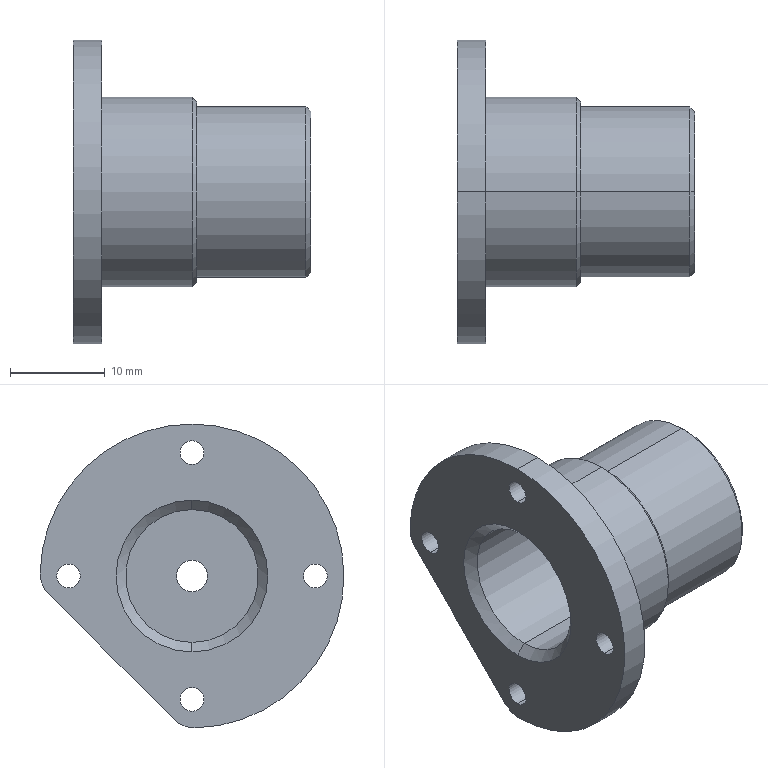Part | SolidWorks | features Chamfer 2, HoleWzd 2, ICE 2, 3DProfileFeature 1, Fillet 1, Revolution 1 | 1 solid | 37 faces | box 25 x 31.997 x 31.997 mm | volume 4923 mm3 | cylinder 22 | cone 8 | plane 7 | commonest cylinder face diameters 2.5 x8 14 x4 3.3 x2 6 x2 18 x2 20 x2
STEP:
#1=CARTESIAN_POINT('',(1.,0.,-7.));
#2=VERTEX_POINT('',#1);
#3=CARTESIAN_POINT('',(1.,0.,7.));
#4=VERTEX_POINT('',#3);
#5=CARTESIAN_POINT('',(1.,0.,0.));
#6=DIRECTION('',(-1.,0.,0.));
#7=DIRECTION('',(0.,0.,-1.));
#8=AXIS2_PLACEMENT_3D('',#5,#6,#7);
#9=CIRCLE('',#8,7.);
#10=EDGE_CURVE('',#2,#4,#9,.T.);
#11=ORIENTED_EDGE('',*,*,#10,.F.);
#12=CARTESIAN_POINT('',(0.,0.,-8.));
#13=VERTEX_POINT('',#12);
#14=CARTESIAN_POINT('',(1.,0.,-7.));
#15=DIRECTION('',(-0.7071,0.,-0.7071));
#16=VECTOR('',#15,1000.);
#17=LINE('',#14,#16);
#18=EDGE_CURVE('',#2,#13,#17,.T.);
#19=ORIENTED_EDGE('',*,*,#18,.T.);
#20=CARTESIAN_POINT('',(0.,0.,8.));
#21=VERTEX_POINT('',#20);
#22=CARTESIAN_POINT('',(0.,0.,0.));
#23=DIRECTION('',(1.,0.,0.));
#24=DIRECTION('',(0.,0.,-1.));
#25=AXIS2_PLACEMENT_3D('',#22,#23,#24);
#26=CIRCLE('',#25,8.);
#27=EDGE_CURVE('',#21,#13,#26,.T.);
#28=ORIENTED_EDGE('',*,*,#27,.F.);
#29=CARTESIAN_POINT('',(1.,0.,7.));
#30=DIRECTION('',(-0.7071,0.,0.7071));
#31=VECTOR('',#30,1000.);
#32=LINE('',#29,#31);
#33=EDGE_CURVE('',#4,#21,#32,.T.);
#34=ORIENTED_EDGE('',*,*,#33,.F.);
#35=EDGE_LOOP('',(#11,#19,#28,#34));
#36=FACE_OUTER_BOUND('',#35,.T.);
#37=CARTESIAN_POINT('',(1.,0.,0.));
#38=DIRECTION('',(-1.,0.,0.));
#39=DIRECTION('',(0.,0.,1.));
#40=AXIS2_PLACEMENT_3D('',#37,#38,#39);
#41=CONICAL_SURFACE('',#40,7.,0.7854);
#42=ADVANCED_FACE('',(#36),#41,.F.);
#43=CARTESIAN_POINT('',(25.,0.,-8.5));
#44=VERTEX_POINT('',#43);
#45=CARTESIAN_POINT('',(25.,0.,8.5));
#46=VERTEX_POINT('',#45);
#47=CARTESIAN_POINT('',(25.,0.,0.));
#48=DIRECTION('',(1.,0.,0.));
#49=DIRECTION('',(0.,0.,1.));
#50=AXIS2_PLACEMENT_3D('',#47,#48,#49);
#51=CIRCLE('',#50,8.5);
#52=EDGE_CURVE('',#44,#46,#51,.T.);
#53=ORIENTED_EDGE('',*,*,#52,.F.);
#54=CARTESIAN_POINT('',(24.5,0.,-9.));
#55=VERTEX_POINT('',#54);
#56=CARTESIAN_POINT('',(24.5,0.,-9.));
#57=DIRECTION('',(-0.7071,0.,-0.7071));
#58=VECTOR('',#57,1000.);
#59=LINE('',#56,#58);
#60=EDGE_CURVE('',#44,#55,#59,.T.);
#61=ORIENTED_EDGE('',*,*,#60,.T.);
#62=CARTESIAN_POINT('',(24.5,0.,9.));
#63=VERTEX_POINT('',#62);
#64=CARTESIAN_POINT('',(24.5,0.,0.));
#65=DIRECTION('',(-1.,0.,0.));
#66=DIRECTION('',(0.,0.,1.));
#67=AXIS2_PLACEMENT_3D('',#64,#65,#66);
#68=CIRCLE('',#67,9.);
#69=EDGE_CURVE('',#63,#55,#68,.T.);
#70=ORIENTED_EDGE('',*,*,#69,.F.);
#71=CARTESIAN_POINT('',(24.5,0.,9.));
#72=DIRECTION('',(-0.7071,0.,0.7071));
#73=VECTOR('',#72,1000.);
#74=LINE('',#71,#73);
#75=EDGE_CURVE('',#46,#63,#74,.T.);
#76=ORIENTED_EDGE('',*,*,#75,.F.);
#77=EDGE_LOOP('',(#53,#61,#70,#76));
#78=FACE_OUTER_BOUND('',#77,.T.);
#79=CARTESIAN_POINT('',(24.5,0.,0.));
#80=DIRECTION('',(-1.,0.,0.));
#81=DIRECTION('',(0.,0.,1.));
#82=AXIS2_PLACEMENT_3D('',#79,#80,#81);
#83=CONICAL_SURFACE('',#82,9.,0.7854);
#84=ADVANCED_FACE('',(#78),#83,.T.);
#85=CARTESIAN_POINT('',(13.,0.,-9.5));
#86=VERTEX_POINT('',#85);
#87=CARTESIAN_POINT('',(13.,0.,9.5));
#88=VERTEX_POINT('',#87);
#89=CARTESIAN_POINT('',(13.,0.,0.));
#90=DIRECTION('',(1.,0.,0.));
#91=DIRECTION('',(0.,0.,1.));
#92=AXIS2_PLACEMENT_3D('',#89,#90,#91);
#93=CIRCLE('',#92,9.5);
#94=EDGE_CURVE('',#86,#88,#93,.T.);
#95=ORIENTED_EDGE('',*,*,#94,.F.);
#96=CARTESIAN_POINT('',(12.5,0.,-10.));
#97=VERTEX_POINT('',#96);
#98=CARTESIAN_POINT('',(12.5,0.,-10.));
#99=DIRECTION('',(-0.7071,0.,-0.7071));
#100=VECTOR('',#99,1000.);
#101=LINE('',#98,#100);
#102=EDGE_CURVE('',#86,#97,#101,.T.);
#103=ORIENTED_EDGE('',*,*,#102,.T.);
#104=CARTESIAN_POINT('',(12.5,0.,10.));
#105=VERTEX_POINT('',#104);
#106=CARTESIAN_POINT('',(12.5,0.,0.));
#107=DIRECTION('',(-1.,0.,0.));
#108=DIRECTION('',(0.,0.,1.));
#109=AXIS2_PLACEMENT_3D('',#106,#107,#108);
#110=CIRCLE('',#109,10.);
#111=EDGE_CURVE('',#105,#97,#110,.T.);
#112=ORIENTED_EDGE('',*,*,#111,.F.);
#113=CARTESIAN_POINT('',(12.5,0.,10.));
#114=DIRECTION('',(-0.7071,0.,0.7071));
#115=VECTOR('',#114,1000.);
#116=LINE('',#113,#115);
#117=EDGE_CURVE('',#88,#105,#116,.T.);
#118=ORIENTED_EDGE('',*,*,#117,.F.);
#119=EDGE_LOOP('',(#95,#103,#112,#118));
#120=FACE_OUTER_BOUND('',#119,.T.);
#121=CARTESIAN_POINT('',(12.5,0.,0.));
#122=DIRECTION('',(-1.,0.,0.));
#123=DIRECTION('',(0.,0.,1.));
#124=AXIS2_PLACEMENT_3D('',#121,#122,#123);
#125=CONICAL_SURFACE('',#124,10.,0.7854);
#126=ADVANCED_FACE('',(#120),#125,.T.);
#127=CARTESIAN_POINT('',(21.625,0.,1.65));
#128=VERTEX_POINT('',#127);
#129=CARTESIAN_POINT('',(21.625,0.,-1.65));
#130=VERTEX_POINT('',#129);
#131=CARTESIAN_POINT('',(21.625,0.,0.));
#132=DIRECTION('',(1.,0.,0.));
#133=DIRECTION('',(0.,0.,-1.));
#134=AXIS2_PLACEMENT_3D('',#131,#132,#133);
#135=CIRCLE('',#134,1.65);
#136=EDGE_CURVE('',#128,#130,#135,.T.);
#137=ORIENTED_EDGE('',*,*,#136,.F.);
#138=CARTESIAN_POINT('',(22.,0.,2.025));
#139=VERTEX_POINT('',#138);
#140=CARTESIAN_POINT('',(22.,0.,2.025));
#141=DIRECTION('',(0.7071,0.,0.7071));
#142=VECTOR('',#141,1000.);
#143=LINE('',#140,#142);
#144=EDGE_CURVE('',#128,#139,#143,.T.);
#145=ORIENTED_EDGE('',*,*,#144,.T.);
#146=CARTESIAN_POINT('',(22.,0.,-2.025));
#147=VERTEX_POINT('',#146);
#148=CARTESIAN_POINT('',(22.,0.,0.));
#149=DIRECTION('',(1.,0.,0.));
#150=DIRECTION('',(0.,0.,-1.));
#151=AXIS2_PLACEMENT_3D('',#148,#149,#150);
#152=CIRCLE('',#151,2.025);
#153=EDGE_CURVE('',#139,#147,#152,.T.);
#154=ORIENTED_EDGE('',*,*,#153,.T.);
#155=CARTESIAN_POINT('',(22.,0.,-2.025));
#156=DIRECTION('',(0.7071,0.,-0.7071));
#157=VECTOR('',#156,1000.);
#158=LINE('',#155,#157);
#159=EDGE_CURVE('',#130,#147,#158,.T.);
#160=ORIENTED_EDGE('',*,*,#159,.F.);
#161=EDGE_LOOP('',(#137,#145,#154,#160));
#162=FACE_OUTER_BOUND('',#161,.T.);
#163=CARTESIAN_POINT('',(22.,0.,0.));
#164=DIRECTION('',(1.,0.,0.));
#165=DIRECTION('',(0.,0.,-1.));
#166=AXIS2_PLACEMENT_3D('',#163,#164,#165);
#167=CONICAL_SURFACE('',#166,2.025,0.7854);
#168=ADVANCED_FACE('',(#162),#167,.F.);
#169=CARTESIAN_POINT('',(19.,0.,1.65));
#170=VERTEX_POINT('',#169);
#171=CARTESIAN_POINT('',(19.,0.,-1.65));
#172=VERTEX_POINT('',#171);
#173=CARTESIAN_POINT('',(19.,0.,0.));
#174=DIRECTION('',(1.,0.,0.));
#175=DIRECTION('',(0.,0.,-1.));
#176=AXIS2_PLACEMENT_3D('',#173,#174,#175);
#177=CIRCLE('',#176,1.65);
#178=EDGE_CURVE('',#170,#172,#177,.T.);
#179=ORIENTED_EDGE('',*,*,#178,.F.);
#180=CARTESIAN_POINT('',(22.,0.,1.65));
#181=DIRECTION('',(1.,0.,0.));
#182=VECTOR('',#181,1000.);
#183=LINE('',#180,#182);
#184=EDGE_CURVE('',#170,#128,#183,.T.);
#185=ORIENTED_EDGE('',*,*,#184,.T.);
#186=ORIENTED_EDGE('',*,*,#136,.T.);
#187=CARTESIAN_POINT('',(22.,0.,-1.65));
#188=DIRECTION('',(1.,0.,0.));
#189=VECTOR('',#188,1000.);
#190=LINE('',#187,#189);
#191=EDGE_CURVE('',#172,#130,#190,.T.);
#192=ORIENTED_EDGE('',*,*,#191,.F.);
#193=EDGE_LOOP('',(#179,#185,#186,#192));
#194=FACE_OUTER_BOUND('',#193,.T.);
#195=CARTESIAN_POINT('',(22.,0.,0.));
#196=DIRECTION('',(1.,0.,0.));
#197=DIRECTION('',(0.,0.,-1.));
#198=AXIS2_PLACEMENT_3D('',#195,#196,#197);
#199=CYLINDRICAL_SURFACE('',#198,1.65);
#200=ADVANCED_FACE('',(#194),#199,.F.);
#201=CARTESIAN_POINT('',(0.,13.,1.25));
#202=VERTEX_POINT('',#201);
#203=CARTESIAN_POINT('',(0.,13.,-1.25));
#204=VERTEX_POINT('',#203);
#205=CARTESIAN_POINT('',(0.,13.,0.));
#206=DIRECTION('',(1.,0.,0.));
#207=DIRECTION('',(0.,0.,-1.));
#208=AXIS2_PLACEMENT_3D('',#205,#206,#207);
#209=CIRCLE('',#208,1.25);
#210=EDGE_CURVE('',#202,#204,#209,.T.);
#211=ORIENTED_EDGE('',*,*,#210,.F.);
#212=CARTESIAN_POINT('',(3.,13.,1.25));
#213=VERTEX_POINT('',#212);
#214=CARTESIAN_POINT('',(0.,13.,1.25));
#215=DIRECTION('',(1.,0.,0.));
#216=VECTOR('',#215,1000.);
#217=LINE('',#214,#216);
#218=EDGE_CURVE('',#202,#213,#217,.T.);
#219=ORIENTED_EDGE('',*,*,#218,.T.);
#220=CARTESIAN_POINT('',(3.,13.,-1.25));
#221=VERTEX_POINT('',#220);
#222=CARTESIAN_POINT('',(3.,13.,0.));
#223=DIRECTION('',(1.,0.,0.));
#224=DIRECTION('',(0.,0.,-1.));
#225=AXIS2_PLACEMENT_3D('',#222,#223,#224);
#226=CIRCLE('',#225,1.25);
#227=EDGE_CURVE('',#213,#221,#226,.T.);
#228=ORIENTED_EDGE('',*,*,#227,.T.);
#229=CARTESIAN_POINT('',(0.,13.,-1.25));
#230=DIRECTION('',(1.,0.,0.));
#231=VECTOR('',#230,1000.);
#232=LINE('',#229,#231);
#233=EDGE_CURVE('',#204,#221,#232,.T.);
#234=ORIENTED_EDGE('',*,*,#233,.F.);
#235=EDGE_LOOP('',(#211,#219,#228,#234));
#236=FACE_OUTER_BOUND('',#235,.T.);
#237=CARTESIAN_POINT('',(0.,13.,0.));
#238=DIRECTION('',(1.,0.,0.));
#239=DIRECTION('',(0.,0.,-1.));
#240=AXIS2_PLACEMENT_3D('',#237,#238,#239);
#241=CYLINDRICAL_SURFACE('',#240,1.25);
#242=ADVANCED_FACE('',(#236),#241,.F.);
#243=CARTESIAN_POINT('',(0.,0.,-11.75));
#244=VERTEX_POINT('',#243);
#245=CARTESIAN_POINT('',(0.,0.,-14.25));
#246=VERTEX_POINT('',#245);
#247=CARTESIAN_POINT('',(0.,0.,-13.));
#248=DIRECTION('',(1.,0.,0.));
#249=DIRECTION('',(0.,0.,-1.));
#250=AXIS2_PLACEMENT_3D('',#247,#248,#249);
#251=CIRCLE('',#250,1.25);
#252=EDGE_CURVE('',#244,#246,#251,.T.);
#253=ORIENTED_EDGE('',*,*,#252,.F.);
#254=CARTESIAN_POINT('',(3.,0.,-11.75));
#255=VERTEX_POINT('',#254);
#256=CARTESIAN_POINT('',(0.,0.,-11.75));
#257=DIRECTION('',(1.,0.,0.));
#258=VECTOR('',#257,1000.);
#259=LINE('',#256,#258);
#260=EDGE_CURVE('',#244,#255,#259,.T.);
#261=ORIENTED_EDGE('',*,*,#260,.T.);
#262=CARTESIAN_POINT('',(3.,0.,-14.25));
#263=VERTEX_POINT('',#262);
#264=CARTESIAN_POINT('',(3.,0.,-13.));
#265=DIRECTION('',(1.,0.,0.));
#266=DIRECTION('',(0.,0.,-1.));
#267=AXIS2_PLACEMENT_3D('',#264,#265,#266);
#268=CIRCLE('',#267,1.25);
#269=EDGE_CURVE('',#255,#263,#268,.T.);
#270=ORIENTED_EDGE('',*,*,#269,.T.);
#271=CARTESIAN_POINT('',(0.,0.,-14.25));
#272=DIRECTION('',(1.,0.,0.));
#273=VECTOR('',#272,1000.);
#274=LINE('',#271,#273);
#275=EDGE_CURVE('',#246,#263,#274,.T.);
#276=ORIENTED_EDGE('',*,*,#275,.F.);
#277=EDGE_LOOP('',(#253,#261,#270,#276));
#278=FACE_OUTER_BOUND('',#277,.T.);
#279=CARTESIAN_POINT('',(0.,0.,-13.));
#280=DIRECTION('',(1.,0.,0.));
#281=DIRECTION('',(0.,0.,-1.));
#282=AXIS2_PLACEMENT_3D('',#279,#280,#281);
#283=CYLINDRICAL_SURFACE('',#282,1.25);
#284=ADVANCED_FACE('',(#278),#283,.F.);
#285=CARTESIAN_POINT('',(0.,-13.,1.25));
#286=VERTEX_POINT('',#285);
#287=CARTESIAN_POINT('',(0.,-13.,-1.25));
#288=VERTEX_POINT('',#287);
#289=CARTESIAN_POINT('',(0.,-13.,0.));
#290=DIRECTION('',(1.,0.,0.));
#291=DIRECTION('',(0.,0.,-1.));
#292=AXIS2_PLACEMENT_3D('',#289,#290,#291);
#293=CIRCLE('',#292,1.25);
#294=EDGE_CURVE('',#286,#288,#293,.T.);
#295=ORIENTED_EDGE('',*,*,#294,.F.);
#296=CARTESIAN_POINT('',(3.,-13.,1.25));
#297=VERTEX_POINT('',#296);
#298=CARTESIAN_POINT('',(0.,-13.,1.25));
#299=DIRECTION('',(1.,0.,0.));
#300=VECTOR('',#299,1000.);
#301=LINE('',#298,#300);
#302=EDGE_CURVE('',#286,#297,#301,.T.);
#303=ORIENTED_EDGE('',*,*,#302,.T.);
#304=CARTESIAN_POINT('',(3.,-13.,-1.25));
#305=VERTEX_POINT('',#304);
#306=CARTESIAN_POINT('',(3.,-13.,0.));
#307=DIRECTION('',(1.,0.,0.));
#308=DIRECTION('',(0.,0.,-1.));
#309=AXIS2_PLACEMENT_3D('',#306,#307,#308);
#310=CIRCLE('',#309,1.25);
#311=EDGE_CURVE('',#297,#305,#310,.T.);
#312=ORIENTED_EDGE('',*,*,#311,.T.);
#313=CARTESIAN_POINT('',(0.,-13.,-1.25));
#314=DIRECTION('',(1.,0.,0.));
#315=VECTOR('',#314,1000.);
#316=LINE('',#313,#315);
#317=EDGE_CURVE('',#288,#305,#316,.T.);
#318=ORIENTED_EDGE('',*,*,#317,.F.);
#319=EDGE_LOOP('',(#295,#303,#312,#318));
#320=FACE_OUTER_BOUND('',#319,.T.);
#321=CARTESIAN_POINT('',(0.,-13.,0.));
#322=DIRECTION('',(1.,0.,0.));
#323=DIRECTION('',(0.,0.,-1.));
#324=AXIS2_PLACEMENT_3D('',#321,#322,#323);
#325=CYLINDRICAL_SURFACE('',#324,1.25);
#326=ADVANCED_FACE('',(#320),#325,.F.);
#327=CARTESIAN_POINT('',(0.,0.,14.25));
#328=VERTEX_POINT('',#327);
#329=CARTESIAN_POINT('',(0.,0.,11.75));
#330=VERTEX_POINT('',#329);
#331=CARTESIAN_POINT('',(0.,0.,13.));
#332=DIRECTION('',(1.,0.,0.));
#333=DIRECTION('',(0.,0.,-1.));
#334=AXIS2_PLACEMENT_3D('',#331,#332,#333);
#335=CIRCLE('',#334,1.25);
#336=EDGE_CURVE('',#328,#330,#335,.T.);
#337=ORIENTED_EDGE('',*,*,#336,.F.);
#338=CARTESIAN_POINT('',(3.,0.,14.25));
#339=VERTEX_POINT('',#338);
#340=CARTESIAN_POINT('',(0.,0.,14.25));
#341=DIRECTION('',(1.,0.,0.));
#342=VECTOR('',#341,1000.);
#343=LINE('',#340,#342);
#344=EDGE_CURVE('',#328,#339,#343,.T.);
#345=ORIENTED_EDGE('',*,*,#344,.T.);
#346=CARTESIAN_POINT('',(3.,0.,11.75));
#347=VERTEX_POINT('',#346);
#348=CARTESIAN_POINT('',(3.,0.,13.));
#349=DIRECTION('',(1.,0.,0.));
#350=DIRECTION('',(0.,0.,-1.));
#351=AXIS2_PLACEMENT_3D('',#348,#349,#350);
#352=CIRCLE('',#351,1.25);
#353=EDGE_CURVE('',#339,#347,#352,.T.);
#354=ORIENTED_EDGE('',*,*,#353,.T.);
#355=CARTESIAN_POINT('',(0.,0.,11.75));
#356=DIRECTION('',(1.,0.,0.));
#357=VECTOR('',#356,1000.);
#358=LINE('',#355,#357);
#359=EDGE_CURVE('',#330,#347,#358,.T.);
#360=ORIENTED_EDGE('',*,*,#359,.F.);
#361=EDGE_LOOP('',(#337,#345,#354,#360));
#362=FACE_OUTER_BOUND('',#361,.T.);
#363=CARTESIAN_POINT('',(0.,0.,13.));
#364=DIRECTION('',(1.,0.,0.));
#365=DIRECTION('',(0.,0.,-1.));
#366=AXIS2_PLACEMENT_3D('',#363,#364,#365);
#367=CYLINDRICAL_SURFACE('',#366,1.25);
#368=ADVANCED_FACE('',(#362),#367,.F.);
#369=CARTESIAN_POINT('',(25.,0.,-7.));
#370=VERTEX_POINT('',#369);
#371=CARTESIAN_POINT('',(25.,0.,7.));
#372=VERTEX_POINT('',#371);
#373=CARTESIAN_POINT('',(25.,0.,0.));
#374=DIRECTION('',(-1.,0.,0.));
#375=DIRECTION('',(0.,0.,1.));
#376=AXIS2_PLACEMENT_3D('',#373,#374,#375);
#377=CIRCLE('',#376,7.);
#378=EDGE_CURVE('',#370,#372,#377,.T.);
#379=ORIENTED_EDGE('',*,*,#378,.F.);
#380=CARTESIAN_POINT('',(22.,0.,-7.));
#381=VERTEX_POINT('',#380);
#382=CARTESIAN_POINT('',(-407.868,0.,-7.));
#383=DIRECTION('',(-1.,0.,0.));
#384=VECTOR('',#383,1000.);
#385=LINE('',#382,#384);
#386=EDGE_CURVE('',#370,#381,#385,.T.);
#387=ORIENTED_EDGE('',*,*,#386,.T.);
#388=CARTESIAN_POINT('',(22.,0.,7.));
#389=VERTEX_POINT('',#388);
#390=CARTESIAN_POINT('',(22.,0.,0.));
#391=DIRECTION('',(-1.,0.,0.));
#392=DIRECTION('',(0.,0.,1.));
#393=AXIS2_PLACEMENT_3D('',#390,#391,#392);
#394=CIRCLE('',#393,7.);
#395=EDGE_CURVE('',#381,#389,#394,.T.);
#396=ORIENTED_EDGE('',*,*,#395,.T.);
#397=CARTESIAN_POINT('',(-407.868,0.,7.));
#398=DIRECTION('',(-1.,0.,0.));
#399=VECTOR('',#398,1000.);
#400=LINE('',#397,#399);
#401=EDGE_CURVE('',#372,#389,#400,.T.);
#402=ORIENTED_EDGE('',*,*,#401,.F.);
#403=EDGE_LOOP('',(#379,#387,#396,#402));
#404=FACE_OUTER_BOUND('',#403,.T.);
#405=CARTESIAN_POINT('',(-407.868,0.,0.));
#406=DIRECTION('',(-1.,0.,0.));
#407=DIRECTION('',(0.,0.,1.));
#408=AXIS2_PLACEMENT_3D('',#405,#406,#407);
#409=CYLINDRICAL_SURFACE('',#408,7.);
#410=ADVANCED_FACE('',(#404),#409,.F.);
#411=ORIENTED_EDGE('',*,*,#69,.T.);
#412=CARTESIAN_POINT('',(13.,0.,-9.));
#413=VERTEX_POINT('',#412);
#414=CARTESIAN_POINT('',(-407.868,0.,-9.));
#415=DIRECTION('',(-1.,0.,0.));
#416=VECTOR('',#415,1000.);
#417=LINE('',#414,#416);
#418=EDGE_CURVE('',#55,#413,#417,.T.);
#419=ORIENTED_EDGE('',*,*,#418,.T.);
#420=CARTESIAN_POINT('',(13.,0.,9.));
#421=VERTEX_POINT('',#420);
#422=CARTESIAN_POINT('',(13.,0.,0.));
#423=DIRECTION('',(-1.,0.,0.));
#424=DIRECTION('',(0.,0.,1.));
#425=AXIS2_PLACEMENT_3D('',#422,#423,#424);
#426=CIRCLE('',#425,9.);
#427=EDGE_CURVE('',#421,#413,#426,.T.);
#428=ORIENTED_EDGE('',*,*,#427,.F.);
#429=CARTESIAN_POINT('',(-407.868,0.,9.));
#430=DIRECTION('',(-1.,0.,0.));
#431=VECTOR('',#430,1000.);
#432=LINE('',#429,#431);
#433=EDGE_CURVE('',#63,#421,#432,.T.);
#434=ORIENTED_EDGE('',*,*,#433,.F.);
#435=EDGE_LOOP('',(#411,#419,#428,#434));
#436=FACE_OUTER_BOUND('',#435,.T.);
#437=CARTESIAN_POINT('',(-407.868,0.,0.));
#438=DIRECTION('',(-1.,0.,0.));
#439=DIRECTION('',(0.,0.,1.));
#440=AXIS2_PLACEMENT_3D('',#437,#438,#439);
#441=CYLINDRICAL_SURFACE('',#440,9.);
#442=ADVANCED_FACE('',(#436),#441,.T.);
#443=ORIENTED_EDGE('',*,*,#111,.T.);
#444=CARTESIAN_POINT('',(3.,0.,-10.));
#445=VERTEX_POINT('',#444);
#446=CARTESIAN_POINT('',(-407.868,0.,-10.));
#447=DIRECTION('',(-1.,0.,0.));
#448=VECTOR('',#447,1000.);
#449=LINE('',#446,#448);
#450=EDGE_CURVE('',#97,#445,#449,.T.);
#451=ORIENTED_EDGE('',*,*,#450,.T.);
#452=CARTESIAN_POINT('',(3.,0.,10.));
#453=VERTEX_POINT('',#452);
#454=CARTESIAN_POINT('',(3.,0.,0.));
#455=DIRECTION('',(-1.,0.,0.));
#456=DIRECTION('',(0.,0.,1.));
#457=AXIS2_PLACEMENT_3D('',#454,#455,#456);
#458=CIRCLE('',#457,10.);
#459=EDGE_CURVE('',#453,#445,#458,.T.);
#460=ORIENTED_EDGE('',*,*,#459,.F.);
#461=CARTESIAN_POINT('',(-407.868,0.,10.));
#462=DIRECTION('',(-1.,0.,0.));
#463=VECTOR('',#462,1000.);
#464=LINE('',#461,#463);
#465=EDGE_CURVE('',#105,#453,#464,.T.);
#466=ORIENTED_EDGE('',*,*,#465,.F.);
#467=EDGE_LOOP('',(#443,#451,#460,#466));
#468=FACE_OUTER_BOUND('',#467,.T.);
#469=CARTESIAN_POINT('',(-407.868,0.,0.));
#470=DIRECTION('',(-1.,0.,0.));
#471=DIRECTION('',(0.,0.,1.));
#472=AXIS2_PLACEMENT_3D('',#469,#470,#471);
#473=CYLINDRICAL_SURFACE('',#472,10.);
#474=ADVANCED_FACE('',(#468),#473,.T.);
#475=CARTESIAN_POINT('',(3.,-0.3314,-15.997));
#476=VERTEX_POINT('',#475);
#477=CARTESIAN_POINT('',(3.,0.,16.));
#478=VERTEX_POINT('',#477);
#479=CARTESIAN_POINT('',(3.,0.,0.));
#480=DIRECTION('',(-1.,0.,0.));
#481=DIRECTION('',(0.,0.,1.));
#482=AXIS2_PLACEMENT_3D('',#479,#480,#481);
#483=CIRCLE('',#482,16.);
#484=EDGE_CURVE('',#476,#478,#483,.T.);
#485=ORIENTED_EDGE('',*,*,#484,.T.);
#486=CARTESIAN_POINT('',(0.,0.,16.));
#487=VERTEX_POINT('',#486);
#488=CARTESIAN_POINT('',(-407.868,0.,16.));
#489=DIRECTION('',(-1.,0.,0.));
#490=VECTOR('',#489,1000.);
#491=LINE('',#488,#490);
#492=EDGE_CURVE('',#478,#487,#491,.T.);
#493=ORIENTED_EDGE('',*,*,#492,.T.);
#494=CARTESIAN_POINT('',(0.,-0.3314,-15.997));
#495=VERTEX_POINT('',#494);
#496=CARTESIAN_POINT('',(0.,0.,0.));
#497=DIRECTION('',(-1.,0.,0.));
#498=DIRECTION('',(0.,0.,1.));
#499=AXIS2_PLACEMENT_3D('',#496,#497,#498);
#500=CIRCLE('',#499,16.);
#501=EDGE_CURVE('',#495,#487,#500,.T.);
#502=ORIENTED_EDGE('',*,*,#501,.F.);
#503=CARTESIAN_POINT('',(-407.868,-0.3314,-15.997));
#504=DIRECTION('',(1.,0.,0.));
#505=VECTOR('',#504,1000.);
#506=LINE('',#503,#505);
#507=EDGE_CURVE('',#495,#476,#506,.T.);
#508=ORIENTED_EDGE('',*,*,#507,.T.);
#509=EDGE_LOOP('',(#485,#493,#502,#508));
#510=FACE_OUTER_BOUND('',#509,.T.);
#511=CARTESIAN_POINT('',(-407.868,0.,0.));
#512=DIRECTION('',(-1.,0.,0.));
#513=DIRECTION('',(0.,0.,1.));
#514=AXIS2_PLACEMENT_3D('',#511,#512,#513);
#515=CYLINDRICAL_SURFACE('',#514,16.);
#516=ADVANCED_FACE('',(#510),#515,.T.);
#517=CARTESIAN_POINT('',(19.,0.,-7.));
#518=VERTEX_POINT('',#517);
#519=CARTESIAN_POINT('',(19.,0.,7.));
#520=VERTEX_POINT('',#519);
#521=CARTESIAN_POINT('',(19.,0.,0.));
#522=DIRECTION('',(-1.,0.,0.));
#523=DIRECTION('',(0.,0.,1.));
#524=AXIS2_PLACEMENT_3D('',#521,#522,#523);
#525=CIRCLE('',#524,7.);
#526=EDGE_CURVE('',#518,#520,#525,.T.);
#527=ORIENTED_EDGE('',*,*,#526,.F.);
#528=CARTESIAN_POINT('',(-407.868,0.,-7.));
#529=DIRECTION('',(-1.,0.,0.));
#530=VECTOR('',#529,1000.);
#531=LINE('',#528,#530);
#532=EDGE_CURVE('',#518,#2,#531,.T.);
#533=ORIENTED_EDGE('',*,*,#532,.T.);
#534=ORIENTED_EDGE('',*,*,#10,.T.);
#535=CARTESIAN_POINT('',(-407.868,0.,7.));
#536=DIRECTION('',(-1.,0.,0.));
#537=VECTOR('',#536,1000.);
#538=LINE('',#535,#537);
#539=EDGE_CURVE('',#520,#4,#538,.T.);
#540=ORIENTED_EDGE('',*,*,#539,.F.);
#541=EDGE_LOOP('',(#527,#533,#534,#540));
#542=FACE_OUTER_BOUND('',#541,.T.);
#543=CARTESIAN_POINT('',(-407.868,0.,0.));
#544=DIRECTION('',(-1.,0.,0.));
#545=DIRECTION('',(0.,0.,1.));
#546=AXIS2_PLACEMENT_3D('',#543,#544,#545);
#547=CYLINDRICAL_SURFACE('',#546,7.);
#548=ADVANCED_FACE('',(#542),#547,.F.);
#549=ORIENTED_EDGE('',*,*,#532,.F.);
#550=CARTESIAN_POINT('',(19.,0.,0.));
#551=DIRECTION('',(-1.,0.,0.));
#552=DIRECTION('',(0.,0.,1.));
#553=AXIS2_PLACEMENT_3D('',#550,#551,#552);
#554=CIRCLE('',#553,7.);
#555=EDGE_CURVE('',#520,#518,#554,.T.);
#556=ORIENTED_EDGE('',*,*,#555,.F.);
#557=ORIENTED_EDGE('',*,*,#539,.T.);
#558=CARTESIAN_POINT('',(1.,0.,0.));
#559=DIRECTION('',(-1.,0.,0.));
#560=DIRECTION('',(0.,0.,-1.));
#561=AXIS2_PLACEMENT_3D('',#558,#559,#560);
#562=CIRCLE('',#561,7.);
#563=EDGE_CURVE('',#4,#2,#562,.T.);
#564=ORIENTED_EDGE('',*,*,#563,.T.);
#565=EDGE_LOOP('',(#549,#556,#557,#564));
#566=FACE_OUTER_BOUND('',#565,.T.);
#567=CARTESIAN_POINT('',(-407.868,0.,0.));
#568=DIRECTION('',(-1.,0.,0.));
#569=DIRECTION('',(0.,0.,1.));
#570=AXIS2_PLACEMENT_3D('',#567,#568,#569);
#571=CYLINDRICAL_SURFACE('',#570,7.);
#572=ADVANCED_FACE('',(#566),#571,.F.);
#573=ORIENTED_EDGE('',*,*,#27,.T.);
#574=CARTESIAN_POINT('',(0.,0.,0.));
#575=DIRECTION('',(1.,0.,0.));
#576=DIRECTION('',(0.,0.,-1.));
#577=AXIS2_PLACEMENT_3D('',#574,#575,#576);
#578=CIRCLE('',#577,8.);
#579=EDGE_CURVE('',#13,#21,#578,.T.);
#580=ORIENTED_EDGE('',*,*,#579,.T.);
#581=EDGE_LOOP('',(#573,#580));
#582=FACE_BOUND('',#581,.T.);
#583=CARTESIAN_POINT('',(0.,13.,0.));
#584=DIRECTION('',(1.,0.,0.));
#585=DIRECTION('',(0.,0.,-1.));
#586=AXIS2_PLACEMENT_3D('',#583,#584,#585);
#587=CIRCLE('',#586,1.25);
#588=EDGE_CURVE('',#204,#202,#587,.T.);
#589=ORIENTED_EDGE('',*,*,#588,.T.);
#590=ORIENTED_EDGE('',*,*,#210,.T.);
#591=EDGE_LOOP('',(#589,#590));
#592=FACE_BOUND('',#591,.T.);
#593=CARTESIAN_POINT('',(0.,0.,-13.));
#594=DIRECTION('',(1.,0.,0.));
#595=DIRECTION('',(0.,0.,-1.));
#596=AXIS2_PLACEMENT_3D('',#593,#594,#595);
#597=CIRCLE('',#596,1.25);
#598=EDGE_CURVE('',#246,#244,#597,.T.);
#599=ORIENTED_EDGE('',*,*,#598,.T.);
#600=ORIENTED_EDGE('',*,*,#252,.T.);
#601=EDGE_LOOP('',(#599,#600));
#602=FACE_BOUND('',#601,.T.);
#603=CARTESIAN_POINT('',(0.,-13.,0.));
#604=DIRECTION('',(1.,0.,0.));
#605=DIRECTION('',(0.,0.,-1.));
#606=AXIS2_PLACEMENT_3D('',#603,#604,#605);
#607=CIRCLE('',#606,1.25);
#608=EDGE_CURVE('',#288,#286,#607,.T.);
#609=ORIENTED_EDGE('',*,*,#608,.T.);
#610=ORIENTED_EDGE('',*,*,#294,.T.);
#611=EDGE_LOOP('',(#609,#610));
#612=FACE_BOUND('',#611,.T.);
#613=CARTESIAN_POINT('',(0.,0.,13.));
#614=DIRECTION('',(1.,0.,0.));
#615=DIRECTION('',(0.,0.,-1.));
#616=AXIS2_PLACEMENT_3D('',#613,#614,#615);
#617=CIRCLE('',#616,1.25);
#618=EDGE_CURVE('',#330,#328,#617,.T.);
#619=ORIENTED_EDGE('',*,*,#618,.T.);
#620=ORIENTED_EDGE('',*,*,#336,.T.);
#621=EDGE_LOOP('',(#619,#620));
#622=FACE_BOUND('',#621,.T.);
#623=CARTESIAN_POINT('',(0.,15.119,-1.852));
#624=VERTEX_POINT('',#623);
#625=CARTESIAN_POINT('',(0.,1.852,-15.119));
#626=VERTEX_POINT('',#625);
#627=CARTESIAN_POINT('',(0.,4.985,-11.985));
#628=DIRECTION('',(0.,-0.7071,-0.7071));
#629=VECTOR('',#628,1000.);
#630=LINE('',#627,#629);
#631=EDGE_CURVE('',#624,#626,#630,.T.);
#632=ORIENTED_EDGE('',*,*,#631,.T.);
#633=CARTESIAN_POINT('',(0.,-0.2693,-12.997));
#634=DIRECTION('',(-1.,0.,0.));
#635=DIRECTION('',(0.,0.,-1.));
#636=AXIS2_PLACEMENT_3D('',#633,#634,#635);
#637=CIRCLE('',#636,3.);
#638=EDGE_CURVE('',#626,#495,#637,.T.);
#639=ORIENTED_EDGE('',*,*,#638,.T.);
#640=ORIENTED_EDGE('',*,*,#501,.T.);
#641=CARTESIAN_POINT('',(0.,15.997,0.3314));
#642=VERTEX_POINT('',#641);
#643=CARTESIAN_POINT('',(0.,0.,0.));
#644=DIRECTION('',(-1.,0.,0.));
#645=DIRECTION('',(0.,0.,1.));
#646=AXIS2_PLACEMENT_3D('',#643,#644,#645);
#647=CIRCLE('',#646,16.);
#648=EDGE_CURVE('',#487,#642,#647,.T.);
#649=ORIENTED_EDGE('',*,*,#648,.T.);
#650=CARTESIAN_POINT('',(0.,12.997,0.2693));
#651=DIRECTION('',(-1.,0.,0.));
#652=DIRECTION('',(0.,0.,-1.));
#653=AXIS2_PLACEMENT_3D('',#650,#651,#652);
#654=CIRCLE('',#653,3.);
#655=EDGE_CURVE('',#642,#624,#654,.T.);
#656=ORIENTED_EDGE('',*,*,#655,.T.);
#657=EDGE_LOOP('',(#632,#639,#640,#649,#656));
#658=FACE_OUTER_BOUND('',#657,.T.);
#659=CARTESIAN_POINT('',(0.,0.,-7.));
#660=DIRECTION('',(1.,0.,0.));
#661=DIRECTION('',(0.,0.,-1.));
#662=AXIS2_PLACEMENT_3D('',#659,#660,#661);
#663=PLANE('',#662);
#664=ADVANCED_FACE('',(#582,#592,#602,#612,#622,#658),#663,.F.);
#665=ORIENTED_EDGE('',*,*,#492,.F.);
#666=CARTESIAN_POINT('',(3.,15.997,0.3314));
#667=VERTEX_POINT('',#666);
#668=CARTESIAN_POINT('',(3.,0.,0.));
#669=DIRECTION('',(-1.,0.,0.));
#670=DIRECTION('',(0.,0.,1.));
#671=AXIS2_PLACEMENT_3D('',#668,#669,#670);
#672=CIRCLE('',#671,16.);
#673=EDGE_CURVE('',#478,#667,#672,.T.);
#674=ORIENTED_EDGE('',*,*,#673,.T.);
#675=CARTESIAN_POINT('',(-407.868,15.997,0.3314));
#676=DIRECTION('',(-1.,0.,0.));
#677=VECTOR('',#676,1000.);
#678=LINE('',#675,#677);
#679=EDGE_CURVE('',#667,#642,#678,.T.);
#680=ORIENTED_EDGE('',*,*,#679,.T.);
#681=ORIENTED_EDGE('',*,*,#648,.F.);
#682=EDGE_LOOP('',(#665,#674,#680,#681));
#683=FACE_OUTER_BOUND('',#682,.T.);
#684=CARTESIAN_POINT('',(-407.868,0.,0.));
#685=DIRECTION('',(-1.,0.,0.));
#686=DIRECTION('',(0.,0.,1.));
#687=AXIS2_PLACEMENT_3D('',#684,#685,#686);
#688=CYLINDRICAL_SURFACE('',#687,16.);
#689=ADVANCED_FACE('',(#683),#688,.T.);
#690=CARTESIAN_POINT('',(3.,13.,0.));
#691=DIRECTION('',(1.,0.,0.));
#692=DIRECTION('',(0.,0.,-1.));
#693=AXIS2_PLACEMENT_3D('',#690,#691,#692);
#694=CIRCLE('',#693,1.25);
#695=EDGE_CURVE('',#221,#213,#694,.T.);
#696=ORIENTED_EDGE('',*,*,#695,.F.);
#697=ORIENTED_EDGE('',*,*,#227,.F.);
#698=EDGE_LOOP('',(#696,#697));
#699=FACE_BOUND('',#698,.T.);
#700=CARTESIAN_POINT('',(3.,0.,-13.));
#701=DIRECTION('',(1.,0.,0.));
#702=DIRECTION('',(0.,0.,-1.));
#703=AXIS2_PLACEMENT_3D('',#700,#701,#702);
#704=CIRCLE('',#703,1.25);
#705=EDGE_CURVE('',#263,#255,#704,.T.);
#706=ORIENTED_EDGE('',*,*,#705,.F.);
#707=ORIENTED_EDGE('',*,*,#269,.F.);
#708=EDGE_LOOP('',(#706,#707));
#709=FACE_BOUND('',#708,.T.);
#710=CARTESIAN_POINT('',(3.,-13.,0.));
#711=DIRECTION('',(1.,0.,0.));
#712=DIRECTION('',(0.,0.,-1.));
#713=AXIS2_PLACEMENT_3D('',#710,#711,#712);
#714=CIRCLE('',#713,1.25);
#715=EDGE_CURVE('',#305,#297,#714,.T.);
#716=ORIENTED_EDGE('',*,*,#715,.F.);
#717=ORIENTED_EDGE('',*,*,#311,.F.);
#718=EDGE_LOOP('',(#716,#717));
#719=FACE_BOUND('',#718,.T.);
#720=CARTESIAN_POINT('',(3.,0.,13.));
#721=DIRECTION('',(1.,0.,0.));
#722=DIRECTION('',(0.,0.,-1.));
#723=AXIS2_PLACEMENT_3D('',#720,#721,#722);
#724=CIRCLE('',#723,1.25);
#725=EDGE_CURVE('',#347,#339,#724,.T.);
#726=ORIENTED_EDGE('',*,*,#725,.F.);
#727=ORIENTED_EDGE('',*,*,#353,.F.);
#728=EDGE_LOOP('',(#726,#727));
#729=FACE_BOUND('',#728,.T.);
#730=ORIENTED_EDGE('',*,*,#484,.F.);
#731=CARTESIAN_POINT('',(3.,1.852,-15.119));
#732=VERTEX_POINT('',#731);
#733=CARTESIAN_POINT('',(3.,-0.2693,-12.997));
#734=DIRECTION('',(1.,0.,0.));
#735=DIRECTION('',(0.,0.,1.));
#736=AXIS2_PLACEMENT_3D('',#733,#734,#735);
#737=CIRCLE('',#736,3.);
#738=EDGE_CURVE('',#476,#732,#737,.T.);
#739=ORIENTED_EDGE('',*,*,#738,.T.);
#740=CARTESIAN_POINT('',(3.,15.119,-1.852));
#741=VERTEX_POINT('',#740);
#742=CARTESIAN_POINT('',(3.,15.969,-1.002));
#743=DIRECTION('',(0.,-0.7071,-0.7071));
#744=VECTOR('',#743,1000.);
#745=LINE('',#742,#744);
#746=EDGE_CURVE('',#741,#732,#745,.T.);
#747=ORIENTED_EDGE('',*,*,#746,.F.);
#748=CARTESIAN_POINT('',(3.,12.997,0.2693));
#749=DIRECTION('',(1.,0.,0.));
#750=DIRECTION('',(0.,0.,1.));
#751=AXIS2_PLACEMENT_3D('',#748,#749,#750);
#752=CIRCLE('',#751,3.);
#753=EDGE_CURVE('',#741,#667,#752,.T.);
#754=ORIENTED_EDGE('',*,*,#753,.T.);
#755=ORIENTED_EDGE('',*,*,#673,.F.);
#756=EDGE_LOOP('',(#730,#739,#747,#754,#755));
#757=FACE_OUTER_BOUND('',#756,.T.);
#758=ORIENTED_EDGE('',*,*,#459,.T.);
#759=CARTESIAN_POINT('',(3.,0.,0.));
#760=DIRECTION('',(-1.,0.,0.));
#761=DIRECTION('',(0.,0.,1.));
#762=AXIS2_PLACEMENT_3D('',#759,#760,#761);
#763=CIRCLE('',#762,10.);
#764=EDGE_CURVE('',#445,#453,#763,.T.);
#765=ORIENTED_EDGE('',*,*,#764,.T.);
#766=EDGE_LOOP('',(#758,#765));
#767=FACE_BOUND('',#766,.T.);
#768=CARTESIAN_POINT('',(3.,0.,-16.));
#769=DIRECTION('',(-1.,0.,0.));
#770=DIRECTION('',(0.,0.,1.));
#771=AXIS2_PLACEMENT_3D('',#768,#769,#770);
#772=PLANE('',#771);
#773=ADVANCED_FACE('',(#699,#709,#719,#729,#757,#767),#772,.F.);
#774=ORIENTED_EDGE('',*,*,#450,.F.);
#775=CARTESIAN_POINT('',(12.5,0.,0.));
#776=DIRECTION('',(-1.,0.,0.));
#777=DIRECTION('',(0.,0.,1.));
#778=AXIS2_PLACEMENT_3D('',#775,#776,#777);
#779=CIRCLE('',#778,10.);
#780=EDGE_CURVE('',#97,#105,#779,.T.);
#781=ORIENTED_EDGE('',*,*,#780,.T.);
#782=ORIENTED_EDGE('',*,*,#465,.T.);
#783=ORIENTED_EDGE('',*,*,#764,.F.);
#784=EDGE_LOOP('',(#774,#781,#782,#783));
#785=FACE_OUTER_BOUND('',#784,.T.);
#786=CARTESIAN_POINT('',(-407.868,0.,0.));
#787=DIRECTION('',(-1.,0.,0.));
#788=DIRECTION('',(0.,0.,1.));
#789=AXIS2_PLACEMENT_3D('',#786,#787,#788);
#790=CYLINDRICAL_SURFACE('',#789,10.);
#791=ADVANCED_FACE('',(#785),#790,.T.);
#792=CARTESIAN_POINT('',(13.,0.,0.));
#793=DIRECTION('',(1.,0.,0.));
#794=DIRECTION('',(0.,0.,1.));
#795=AXIS2_PLACEMENT_3D('',#792,#793,#794);
#796=CIRCLE('',#795,9.5);
#797=EDGE_CURVE('',#88,#86,#796,.T.);
#798=ORIENTED_EDGE('',*,*,#797,.T.);
#799=ORIENTED_EDGE('',*,*,#94,.T.);
#800=EDGE_LOOP('',(#798,#799));
#801=FACE_OUTER_BOUND('',#800,.T.);
#802=ORIENTED_EDGE('',*,*,#427,.T.);
#803=CARTESIAN_POINT('',(13.,0.,0.));
#804=DIRECTION('',(-1.,0.,0.));
#805=DIRECTION('',(0.,0.,1.));
#806=AXIS2_PLACEMENT_3D('',#803,#804,#805);
#807=CIRCLE('',#806,9.);
#808=EDGE_CURVE('',#413,#421,#807,.T.);
#809=ORIENTED_EDGE('',*,*,#808,.T.);
#810=EDGE_LOOP('',(#802,#809));
#811=FACE_BOUND('',#810,.T.);
#812=CARTESIAN_POINT('',(13.,0.,-10.));
#813=DIRECTION('',(-1.,0.,0.));
#814=DIRECTION('',(0.,0.,1.));
#815=AXIS2_PLACEMENT_3D('',#812,#813,#814);
#816=PLANE('',#815);
#817=ADVANCED_FACE('',(#801,#811),#816,.F.);
#818=ORIENTED_EDGE('',*,*,#418,.F.);
#819=CARTESIAN_POINT('',(24.5,0.,0.));
#820=DIRECTION('',(-1.,0.,0.));
#821=DIRECTION('',(0.,0.,1.));
#822=AXIS2_PLACEMENT_3D('',#819,#820,#821);
#823=CIRCLE('',#822,9.);
#824=EDGE_CURVE('',#55,#63,#823,.T.);
#825=ORIENTED_EDGE('',*,*,#824,.T.);
#826=ORIENTED_EDGE('',*,*,#433,.T.);
#827=ORIENTED_EDGE('',*,*,#808,.F.);
#828=EDGE_LOOP('',(#818,#825,#826,#827));
#829=FACE_OUTER_BOUND('',#828,.T.);
#830=CARTESIAN_POINT('',(-407.868,0.,0.));
#831=DIRECTION('',(-1.,0.,0.));
#832=DIRECTION('',(0.,0.,1.));
#833=AXIS2_PLACEMENT_3D('',#830,#831,#832);
#834=CYLINDRICAL_SURFACE('',#833,9.);
#835=ADVANCED_FACE('',(#829),#834,.T.);
#836=CARTESIAN_POINT('',(25.,0.,0.));
#837=DIRECTION('',(1.,0.,0.));
#838=DIRECTION('',(0.,0.,1.));
#839=AXIS2_PLACEMENT_3D('',#836,#837,#838);
#840=CIRCLE('',#839,8.5);
#841=EDGE_CURVE('',#46,#44,#840,.T.);
#842=ORIENTED_EDGE('',*,*,#841,.T.);
#843=ORIENTED_EDGE('',*,*,#52,.T.);
#844=EDGE_LOOP('',(#842,#843));
#845=FACE_OUTER_BOUND('',#844,.T.);
#846=CARTESIAN_POINT('',(25.,0.,0.));
#847=DIRECTION('',(-1.,0.,0.));
#848=DIRECTION('',(0.,0.,1.));
#849=AXIS2_PLACEMENT_3D('',#846,#847,#848);
#850=CIRCLE('',#849,7.);
#851=EDGE_CURVE('',#372,#370,#850,.T.);
#852=ORIENTED_EDGE('',*,*,#851,.T.);
#853=ORIENTED_EDGE('',*,*,#378,.T.);
#854=EDGE_LOOP('',(#852,#853));
#855=FACE_BOUND('',#854,.T.);
#856=CARTESIAN_POINT('',(25.,0.,-9.));
#857=DIRECTION('',(-1.,0.,0.));
#858=DIRECTION('',(0.,0.,1.));
#859=AXIS2_PLACEMENT_3D('',#856,#857,#858);
#860=PLANE('',#859);
#861=ADVANCED_FACE('',(#845,#855),#860,.F.);
#862=ORIENTED_EDGE('',*,*,#386,.F.);
#863=ORIENTED_EDGE('',*,*,#851,.F.);
#864=ORIENTED_EDGE('',*,*,#401,.T.);
#865=CARTESIAN_POINT('',(22.,0.,0.));
#866=DIRECTION('',(-1.,0.,0.));
#867=DIRECTION('',(0.,0.,1.));
#868=AXIS2_PLACEMENT_3D('',#865,#866,#867);
#869=CIRCLE('',#868,7.);
#870=EDGE_CURVE('',#389,#381,#869,.T.);
#871=ORIENTED_EDGE('',*,*,#870,.T.);
#872=EDGE_LOOP('',(#862,#863,#864,#871));
#873=FACE_OUTER_BOUND('',#872,.T.);
#874=CARTESIAN_POINT('',(-407.868,0.,0.));
#875=DIRECTION('',(-1.,0.,0.));
#876=DIRECTION('',(0.,0.,1.));
#877=AXIS2_PLACEMENT_3D('',#874,#875,#876);
#878=CYLINDRICAL_SURFACE('',#877,7.);
#879=ADVANCED_FACE('',(#873),#878,.F.);
#880=CARTESIAN_POINT('',(22.,0.,0.));
#881=DIRECTION('',(1.,0.,0.));
#882=DIRECTION('',(0.,0.,-1.));
#883=AXIS2_PLACEMENT_3D('',#880,#881,#882);
#884=CIRCLE('',#883,2.025);
#885=EDGE_CURVE('',#147,#139,#884,.T.);
#886=ORIENTED_EDGE('',*,*,#885,.F.);
#887=ORIENTED_EDGE('',*,*,#153,.F.);
#888=EDGE_LOOP('',(#886,#887));
#889=FACE_BOUND('',#888,.T.);
#890=ORIENTED_EDGE('',*,*,#870,.F.);
#891=ORIENTED_EDGE('',*,*,#395,.F.);
#892=EDGE_LOOP('',(#890,#891));
#893=FACE_OUTER_BOUND('',#892,.T.);
#894=CARTESIAN_POINT('',(22.,0.,-7.));
#895=DIRECTION('',(-1.,0.,0.));
#896=DIRECTION('',(0.,0.,1.));
#897=AXIS2_PLACEMENT_3D('',#894,#895,#896);
#898=PLANE('',#897);
#899=ADVANCED_FACE('',(#889,#893),#898,.F.);
#900=CARTESIAN_POINT('',(19.,0.,0.));
#901=DIRECTION('',(1.,0.,0.));
#902=DIRECTION('',(0.,0.,-1.));
#903=AXIS2_PLACEMENT_3D('',#900,#901,#902);
#904=CIRCLE('',#903,1.65);
#905=EDGE_CURVE('',#172,#170,#904,.T.);
#906=ORIENTED_EDGE('',*,*,#905,.T.);
#907=ORIENTED_EDGE('',*,*,#178,.T.);
#908=EDGE_LOOP('',(#906,#907));
#909=FACE_BOUND('',#908,.T.);
#910=ORIENTED_EDGE('',*,*,#555,.T.);
#911=ORIENTED_EDGE('',*,*,#526,.T.);
#912=EDGE_LOOP('',(#910,#911));
#913=FACE_OUTER_BOUND('',#912,.T.);
#914=CARTESIAN_POINT('',(19.,0.,0.));
#915=DIRECTION('',(1.,0.,0.));
#916=DIRECTION('',(0.,0.,-1.));
#917=AXIS2_PLACEMENT_3D('',#914,#915,#916);
#918=PLANE('',#917);
#919=ADVANCED_FACE('',(#909,#913),#918,.F.);
#920=ORIENTED_EDGE('',*,*,#344,.F.);
#921=ORIENTED_EDGE('',*,*,#618,.F.);
#922=ORIENTED_EDGE('',*,*,#359,.T.);
#923=ORIENTED_EDGE('',*,*,#725,.T.);
#924=EDGE_LOOP('',(#920,#921,#922,#923));
#925=FACE_OUTER_BOUND('',#924,.T.);
#926=CARTESIAN_POINT('',(0.,0.,13.));
#927=DIRECTION('',(1.,0.,0.));
#928=DIRECTION('',(0.,0.,-1.));
#929=AXIS2_PLACEMENT_3D('',#926,#927,#928);
#930=CYLINDRICAL_SURFACE('',#929,1.25);
#931=ADVANCED_FACE('',(#925),#930,.F.);
#932=ORIENTED_EDGE('',*,*,#302,.F.);
#933=ORIENTED_EDGE('',*,*,#608,.F.);
#934=ORIENTED_EDGE('',*,*,#317,.T.);
#935=ORIENTED_EDGE('',*,*,#715,.T.);
#936=EDGE_LOOP('',(#932,#933,#934,#935));
#937=FACE_OUTER_BOUND('',#936,.T.);
#938=CARTESIAN_POINT('',(0.,-13.,0.));
#939=DIRECTION('',(1.,0.,0.));
#940=DIRECTION('',(0.,0.,-1.));
#941=AXIS2_PLACEMENT_3D('',#938,#939,#940);
#942=CYLINDRICAL_SURFACE('',#941,1.25);
#943=ADVANCED_FACE('',(#937),#942,.F.);
#944=ORIENTED_EDGE('',*,*,#260,.F.);
#945=ORIENTED_EDGE('',*,*,#598,.F.);
#946=ORIENTED_EDGE('',*,*,#275,.T.);
#947=ORIENTED_EDGE('',*,*,#705,.T.);
#948=EDGE_LOOP('',(#944,#945,#946,#947));
#949=FACE_OUTER_BOUND('',#948,.T.);
#950=CARTESIAN_POINT('',(0.,0.,-13.));
#951=DIRECTION('',(1.,0.,0.));
#952=DIRECTION('',(0.,0.,-1.));
#953=AXIS2_PLACEMENT_3D('',#950,#951,#952);
#954=CYLINDRICAL_SURFACE('',#953,1.25);
#955=ADVANCED_FACE('',(#949),#954,.F.);
#956=ORIENTED_EDGE('',*,*,#218,.F.);
#957=ORIENTED_EDGE('',*,*,#588,.F.);
#958=ORIENTED_EDGE('',*,*,#233,.T.);
#959=ORIENTED_EDGE('',*,*,#695,.T.);
#960=EDGE_LOOP('',(#956,#957,#958,#959));
#961=FACE_OUTER_BOUND('',#960,.T.);
#962=CARTESIAN_POINT('',(0.,13.,0.));
#963=DIRECTION('',(1.,0.,0.));
#964=DIRECTION('',(0.,0.,-1.));
#965=AXIS2_PLACEMENT_3D('',#962,#963,#964);
#966=CYLINDRICAL_SURFACE('',#965,1.25);
#967=ADVANCED_FACE('',(#961),#966,.F.);
#968=ORIENTED_EDGE('',*,*,#184,.F.);
#969=ORIENTED_EDGE('',*,*,#905,.F.);
#970=ORIENTED_EDGE('',*,*,#191,.T.);
#971=CARTESIAN_POINT('',(21.625,0.,0.));
#972=DIRECTION('',(1.,0.,0.));
#973=DIRECTION('',(0.,0.,-1.));
#974=AXIS2_PLACEMENT_3D('',#971,#972,#973);
#975=CIRCLE('',#974,1.65);
#976=EDGE_CURVE('',#130,#128,#975,.T.);
#977=ORIENTED_EDGE('',*,*,#976,.T.);
#978=EDGE_LOOP('',(#968,#969,#970,#977));
#979=FACE_OUTER_BOUND('',#978,.T.);
#980=CARTESIAN_POINT('',(22.,0.,0.));
#981=DIRECTION('',(1.,0.,0.));
#982=DIRECTION('',(0.,0.,-1.));
#983=AXIS2_PLACEMENT_3D('',#980,#981,#982);
#984=CYLINDRICAL_SURFACE('',#983,1.65);
#985=ADVANCED_FACE('',(#979),#984,.F.);
#986=ORIENTED_EDGE('',*,*,#144,.F.);
#987=ORIENTED_EDGE('',*,*,#976,.F.);
#988=ORIENTED_EDGE('',*,*,#159,.T.);
#989=ORIENTED_EDGE('',*,*,#885,.T.);
#990=EDGE_LOOP('',(#986,#987,#988,#989));
#991=FACE_OUTER_BOUND('',#990,.T.);
#992=CARTESIAN_POINT('',(22.,0.,0.));
#993=DIRECTION('',(1.,0.,0.));
#994=DIRECTION('',(0.,0.,-1.));
#995=AXIS2_PLACEMENT_3D('',#992,#993,#994);
#996=CONICAL_SURFACE('',#995,2.025,0.7854);
#997=ADVANCED_FACE('',(#991),#996,.F.);
#998=ORIENTED_EDGE('',*,*,#102,.F.);
#999=ORIENTED_EDGE('',*,*,#797,.F.);
#1000=ORIENTED_EDGE('',*,*,#117,.T.);
#1001=ORIENTED_EDGE('',*,*,#780,.F.);
#1002=EDGE_LOOP('',(#998,#999,#1000,#1001));
#1003=FACE_OUTER_BOUND('',#1002,.T.);
#1004=CARTESIAN_POINT('',(12.5,0.,0.));
#1005=DIRECTION('',(-1.,0.,0.));
#1006=DIRECTION('',(0.,0.,1.));
#1007=AXIS2_PLACEMENT_3D('',#1004,#1005,#1006);
#1008=CONICAL_SURFACE('',#1007,10.,0.7854);
#1009=ADVANCED_FACE('',(#1003),#1008,.T.);
#1010=ORIENTED_EDGE('',*,*,#60,.F.);
#1011=ORIENTED_EDGE('',*,*,#841,.F.);
#1012=ORIENTED_EDGE('',*,*,#75,.T.);
#1013=ORIENTED_EDGE('',*,*,#824,.F.);
#1014=EDGE_LOOP('',(#1010,#1011,#1012,#1013));
#1015=FACE_OUTER_BOUND('',#1014,.T.);
#1016=CARTESIAN_POINT('',(24.5,0.,0.));
#1017=DIRECTION('',(-1.,0.,0.));
#1018=DIRECTION('',(0.,0.,1.));
#1019=AXIS2_PLACEMENT_3D('',#1016,#1017,#1018);
#1020=CONICAL_SURFACE('',#1019,9.,0.7854);
#1021=ADVANCED_FACE('',(#1015),#1020,.T.);
#1022=ORIENTED_EDGE('',*,*,#18,.F.);
#1023=ORIENTED_EDGE('',*,*,#563,.F.);
#1024=ORIENTED_EDGE('',*,*,#33,.T.);
#1025=ORIENTED_EDGE('',*,*,#579,.F.);
#1026=EDGE_LOOP('',(#1022,#1023,#1024,#1025));
#1027=FACE_OUTER_BOUND('',#1026,.T.);
#1028=CARTESIAN_POINT('',(1.,0.,0.));
#1029=DIRECTION('',(-1.,0.,0.));
#1030=DIRECTION('',(0.,0.,1.));
#1031=AXIS2_PLACEMENT_3D('',#1028,#1029,#1030);
#1032=CONICAL_SURFACE('',#1031,7.,0.7854);
#1033=ADVANCED_FACE('',(#1027),#1032,.F.);
#1034=ORIENTED_EDGE('',*,*,#746,.T.);
#1035=CARTESIAN_POINT('',(-7.,1.852,-15.119));
#1036=DIRECTION('',(-1.,0.,0.));
#1037=VECTOR('',#1036,1000.);
#1038=LINE('',#1035,#1037);
#1039=EDGE_CURVE('',#732,#626,#1038,.T.);
#1040=ORIENTED_EDGE('',*,*,#1039,.T.);
#1041=ORIENTED_EDGE('',*,*,#631,.F.);
#1042=CARTESIAN_POINT('',(-7.,15.119,-1.852));
#1043=DIRECTION('',(1.,0.,0.));
#1044=VECTOR('',#1043,1000.);
#1045=LINE('',#1042,#1044);
#1046=EDGE_CURVE('',#624,#741,#1045,.T.);
#1047=ORIENTED_EDGE('',*,*,#1046,.T.);
#1048=EDGE_LOOP('',(#1034,#1040,#1041,#1047));
#1049=FACE_OUTER_BOUND('',#1048,.T.);
#1050=CARTESIAN_POINT('',(-7.,15.969,-1.002));
#1051=DIRECTION('',(0.,-0.7071,0.7071));
#1052=DIRECTION('',(0.,-0.7071,-0.7071));
#1053=AXIS2_PLACEMENT_3D('',#1050,#1051,#1052);
#1054=PLANE('',#1053);
#1055=ADVANCED_FACE('',(#1049),#1054,.F.);
#1056=ORIENTED_EDGE('',*,*,#638,.F.);
#1057=ORIENTED_EDGE('',*,*,#1039,.F.);
#1058=ORIENTED_EDGE('',*,*,#738,.F.);
#1059=ORIENTED_EDGE('',*,*,#507,.F.);
#1060=EDGE_LOOP('',(#1056,#1057,#1058,#1059));
#1061=FACE_OUTER_BOUND('',#1060,.T.);
#1062=CARTESIAN_POINT('',(-407.868,-0.2693,-12.997));
#1063=DIRECTION('',(-1.,0.,0.));
#1064=DIRECTION('',(0.,0.,1.));
#1065=AXIS2_PLACEMENT_3D('',#1062,#1063,#1064);
#1066=CYLINDRICAL_SURFACE('',#1065,3.);
#1067=ADVANCED_FACE('',(#1061),#1066,.T.);
#1068=ORIENTED_EDGE('',*,*,#655,.F.);
#1069=ORIENTED_EDGE('',*,*,#679,.F.);
#1070=ORIENTED_EDGE('',*,*,#753,.F.);
#1071=ORIENTED_EDGE('',*,*,#1046,.F.);
#1072=EDGE_LOOP('',(#1068,#1069,#1070,#1071));
#1073=FACE_OUTER_BOUND('',#1072,.T.);
#1074=CARTESIAN_POINT('',(-407.868,12.997,0.2693));
#1075=DIRECTION('',(-1.,0.,0.));
#1076=DIRECTION('',(0.,0.,1.));
#1077=AXIS2_PLACEMENT_3D('',#1074,#1075,#1076);
#1078=CYLINDRICAL_SURFACE('',#1077,3.);
#1079=ADVANCED_FACE('',(#1073),#1078,.T.);
#1080=CLOSED_SHELL('',(#42,#84,#126,#168,#200,#242,#284,#326,#368,#410,#442,#474,#516,#548,#572,#664,#689,#773,#791,#817,#835,#861,#879,#899,#919,#931,#943,#955,#967,#985,#997,#1009,#1021,#1033,#1055,#1067,#1079));
#1081=MANIFOLD_SOLID_BREP('',#1080);
#1082=CARTESIAN_POINT('',(0.,0.,0.));
#1083=DIRECTION('',(0.,0.,1.));
#1084=DIRECTION('',(1.,0.,0.));
#1085=AXIS2_PLACEMENT_3D('',#1082,#1083,#1084);
#1086=(LENGTH_UNIT()NAMED_UNIT(*)SI_UNIT(.MILLI.,.METRE.));
#1087=UNCERTAINTY_MEASURE_WITH_UNIT(LENGTH_MEASURE(0.00001),#1086,'','');
#1088=(NAMED_UNIT(*)PLANE_ANGLE_UNIT()SI_UNIT($,.RADIAN.));
#1089=(NAMED_UNIT(*)SI_UNIT($,.STERADIAN.)SOLID_ANGLE_UNIT());
#1090=(GEOMETRIC_REPRESENTATION_CONTEXT(3)GLOBAL_UNCERTAINTY_ASSIGNED_CONTEXT((#1087))GLOBAL_UNIT_ASSIGNED_CONTEXT((#1086,#1088,#1089))REPRESENTATION_CONTEXT('',''));
#1091=ADVANCED_BREP_SHAPE_REPRESENTATION('',(#1081,#1085),#1090);